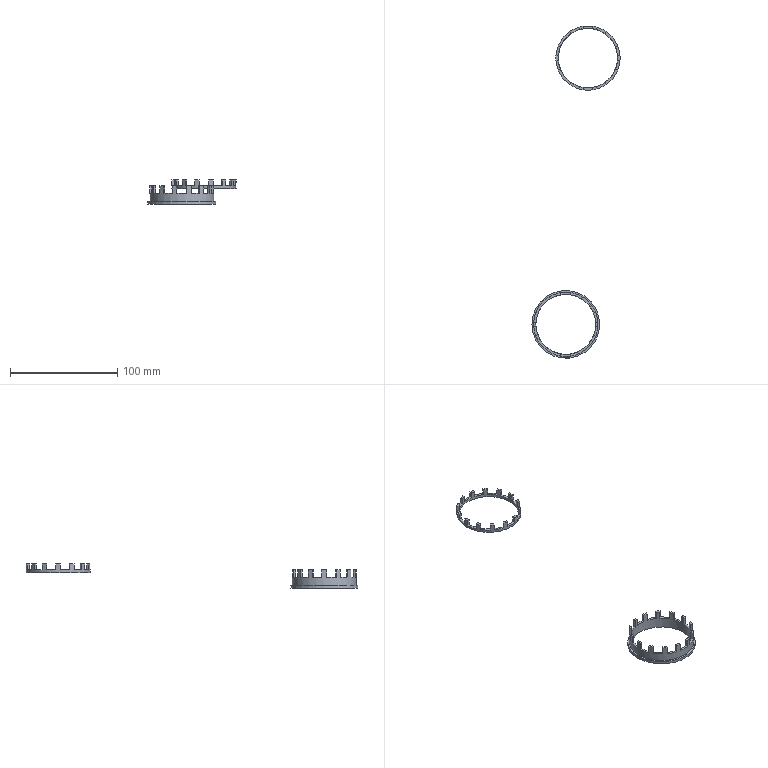NC program | NX | posted with a generic post | part box 82.344 x 310.506 x 22.5 mm
Lines 4390 to 4660 of 4660:
(PLANAR_MILL_1 , TOOL : D2A45)
N8616 T02 M6
N8618 G54
N8620 G17 G0 G90 X3.448 Y-30.698 S9500 M3
N8622 G43 Z30. H2
N8624 Z-6.5
N8626 G94 G1 Z-7.5 F1250.
N8628 G3 X3.321 Y-30.218 R1.
N8630 G2 X-3.321 Y-30.218 R30.4
N8632 G3 X-3.448 Y-30.698 R1.
N8634 G1 Z-6.5
N8636 G0 Z30.
N8638 X-3.183 Y-26.918
N8640 Z-6.5
N8642 G1 Z-7.5
N8644 G3 X-3.189 Y-27.415 R1.
N8646 X3.189 Y-27.415 R27.6
N8648 X3.183 Y-26.918 R1.
N8650 G1 Z-6.5
N8652 G0 Z30.
(PLANAR_MILL_1_COPY , TOOL : D2A45)
N8654 X16.426 Y-26.162
N8656 Z-6.5
N8658 G1 Z-7.5
N8660 G3 X16.103 Y-25.785 R1.
N8662 G2 X10.119 Y-28.666 R30.4
N8664 G3 X10.213 Y-29.154 R1.
N8666 G1 Z-6.5
N8668 G0 Z30.
N8670 X8.812 Y-25.634
N8672 Z-6.5
N8674 G1 Z-7.5
N8676 G3 X9.022 Y-26.084 R1.
N8678 X14.768 Y-23.317 R27.6
N8680 X14.547 Y-22.872 R1.
N8682 G1 Z-6.5
N8684 G0 Z30.
(PLANAR_MILL_1_COPY_1 , TOOL : D2A45)
N8686 X26.151 Y-16.445
N8688 Z-6.5
N8690 G1 Z-7.5
N8692 G3 X25.696 Y-16.244 R1.
N8694 G2 X21.555 Y-21.437 R30.4
N8696 G3 X21.851 Y-21.836 R1.
N8698 G1 Z-6.5
N8700 G0 Z30.
N8702 X19.061 Y-19.272
N8704 Z-6.5
N8706 G1 Z-7.5
N8708 G3 X19.446 Y-19.586 R1.
N8710 X23.422 Y-14.6 R27.6
N8712 X23.03 Y-14.295 R1.
N8714 G1 Z-6.5
N8716 G0 Z30.
(PLANAR_MILL_1_COPY_2 , TOOL : D2A45)
N8718 X30.696 Y-3.47
N8720 Z-6.5
N8722 G1 Z-7.5
N8724 G3 X30.199 Y-3.486 R1.
N8726 G2 X28.721 Y-9.962 R30.4
N8728 G3 X29.162 Y-10.192 R1.
N8730 G1 Z-6.5
N8732 G0 Z30.
N8734 X25.535 Y-9.093
N8736 Z-6.5
N8738 G1 Z-7.5
N8740 G3 X26.018 Y-9.209 R1.
N8742 X27.437 Y-2.992 R27.6
N8744 X26.952 Y-2.887 R1.
N8746 G1 Z-6.5
N8748 G0 Z30.
(PLANAR_MILL_1_COPY_3 , TOOL : D2A45)
N8750 X29.162 Y10.192
N8752 Z-6.5
N8754 G1 Z-7.5
N8756 G3 X28.721 Y9.962 R1.
N8758 G2 X30.199 Y3.486 R30.4
N8760 G3 X30.696 Y3.47 R1.
N8762 G1 Z-6.5
N8764 G0 Z30.
N8766 X26.952 Y2.887
N8768 Z-6.5
N8770 G1 Z-7.5
N8772 G3 X27.437 Y2.992 R1.
N8774 X26.018 Y9.209 R27.6
N8776 X25.535 Y9.093 R1.
N8778 G1 Z-6.5
N8780 G0 Z30.
(PLANAR_MILL_1_COPY_4 , TOOL : D2A45)
N8782 X21.851 Y21.836
N8784 Z-6.5
N8786 G1 Z-7.5
N8788 G3 X21.555 Y21.437 R1.
N8790 G2 X25.696 Y16.244 R30.4
N8792 G3 X26.151 Y16.445 R1.
N8794 G1 Z-6.5
N8796 G0 Z30.
N8798 X23.03 Y14.295
N8800 Z-6.5
N8802 G1 Z-7.5
N8804 G3 X23.422 Y14.6 R1.
N8806 X19.446 Y19.586 R27.6
N8808 X19.061 Y19.272 R1.
N8810 G1 Z-6.5
N8812 G0 Z30.
(PLANAR_MILL_1_COPY_5 , TOOL : D2A45)
N8814 X10.213 Y29.154
N8816 Z-6.5
N8818 G1 Z-7.5
N8820 G3 X10.119 Y28.666 R1.
N8822 G2 X16.103 Y25.785 R30.4
N8824 G3 X16.426 Y26.162 R1.
N8826 G1 Z-6.5
N8828 G0 Z30.
N8830 X14.547 Y22.872
N8832 Z-6.5
N8834 G1 Z-7.5
N8836 G3 X14.768 Y23.317 R1.
N8838 X9.022 Y26.084 R27.6
N8840 X8.812 Y25.634 R1.
N8842 G1 Z-6.5
N8844 G0 Z30.
(PLANAR_MILL_1_COPY_6 , TOOL : D2A45)
N8846 X-3.448 Y30.698
N8848 Z-6.5
N8850 G1 Z-7.5
N8852 G3 X-3.321 Y30.218 R1.
N8854 G2 X3.321 Y30.218 R30.4
N8856 G3 X3.448 Y30.698 R1.
N8858 G1 Z-6.5
N8860 G0 Z30.
N8862 X3.183 Y26.918
N8864 Z-6.5
N8866 G1 Z-7.5
N8868 G3 X3.189 Y27.415 R1.
N8870 X-3.189 Y27.415 R27.6
N8872 X-3.183 Y26.918 R1.
N8874 G1 Z-6.5
N8876 G0 Z30.
(PLANAR_MILL_1_COPY_7 , TOOL : D2A45)
N8878 X-16.426 Y26.162
N8880 Z-6.5
N8882 G1 Z-7.5
N8884 G3 X-16.103 Y25.785 R1.
N8886 G2 X-10.119 Y28.666 R30.4
N8888 G3 X-10.213 Y29.154 R1.
N8890 G1 Z-6.5
N8892 G0 Z30.
N8894 X-8.812 Y25.634
N8896 Z-6.5
N8898 G1 Z-7.5
N8900 G3 X-9.022 Y26.084 R1.
N8902 X-14.768 Y23.317 R27.6
N8904 X-14.547 Y22.872 R1.
N8906 G1 Z-6.5
N8908 G0 Z30.
(PLANAR_MILL_1_COPY_8 , TOOL : D2A45)
N8910 X-26.151 Y16.445
N8912 Z-6.5
N8914 G1 Z-7.5
N8916 G3 X-25.696 Y16.244 R1.
N8918 G2 X-21.555 Y21.437 R30.4
N8920 G3 X-21.851 Y21.836 R1.
N8922 G1 Z-6.5
N8924 G0 Z30.
N8926 X-19.061 Y19.272
N8928 Z-6.5
N8930 G1 Z-7.5
N8932 G3 X-19.446 Y19.586 R1.
N8934 X-23.422 Y14.6 R27.6
N8936 X-23.03 Y14.295 R1.
N8938 G1 Z-6.5
N8940 G0 Z30.
(PLANAR_MILL_1_COPY_9 , TOOL : D2A45)
N8942 X-30.696 Y3.47
N8944 Z-6.5
N8946 G1 Z-7.5
N8948 G3 X-30.199 Y3.486 R1.
N8950 G2 X-28.721 Y9.962 R30.4
N8952 G3 X-29.162 Y10.192 R1.
N8954 G1 Z-6.5
N8956 G0 Z30.
N8958 X-25.535 Y9.093
N8960 Z-6.5
N8962 G1 Z-7.5
N8964 G3 X-26.018 Y9.209 R1.
N8966 X-27.437 Y2.992 R27.6
N8968 X-26.952 Y2.887 R1.
N8970 G1 Z-6.5
N8972 G0 Z30.
(PLANAR_MILL_1_COPY_10 , TOOL : D2A45)
N8974 X-29.162 Y-10.192
N8976 Z-6.5
N8978 G1 Z-7.5
N8980 G3 X-28.721 Y-9.962 R1.
N8982 G2 X-30.199 Y-3.486 R30.4
N8984 G3 X-30.696 Y-3.47 R1.
N8986 G1 Z-6.5
N8988 G0 Z30.
N8990 X-26.952 Y-2.887
N8992 Z-6.5
N8994 G1 Z-7.5
N8996 G3 X-27.437 Y-2.992 R1.
N8998 X-26.018 Y-9.209 R27.6
N9000 X-25.535 Y-9.093 R1.
N9002 G1 Z-6.5
N9004 G0 Z30.
(PLANAR_MILL_1_COPY_11 , TOOL : D2A45)
N9006 X-21.851 Y-21.836
N9008 Z-6.5
N9010 G1 Z-7.5
N9012 G3 X-21.555 Y-21.437 R1.
N9014 G2 X-25.696 Y-16.244 R30.4
N9016 G3 X-26.151 Y-16.445 R1.
N9018 G1 Z-6.5
N9020 G0 Z30.
N9022 X-23.03 Y-14.295
N9024 Z-6.5
N9026 G1 Z-7.5
N9028 G3 X-23.422 Y-14.6 R1.
N9030 X-19.446 Y-19.586 R27.6
N9032 X-19.061 Y-19.272 R1.
N9034 G1 Z-6.5
N9036 G0 Z30.
(PLANAR_MILL_1_COPY_12 , TOOL : D2A45)
N9038 X-10.213 Y-29.154
N9040 Z-6.5
N9042 G1 Z-7.5
N9044 G3 X-10.119 Y-28.666 R1.
N9046 G2 X-16.103 Y-25.785 R30.4
N9048 G3 X-16.426 Y-26.162 R1.
N9050 G1 Z-6.5
N9052 G0 Z30.
N9054 X-14.547 Y-22.872
N9056 Z-6.5
N9058 G1 Z-7.5
N9060 G3 X-14.768 Y-23.317 R1.
N9062 X-9.022 Y-26.084 R27.6
N9064 X-8.812 Y-25.634 R1.
N9066 G1 Z-6.5
N9068 G0 Z30.
N9070 M5
N9072 M2